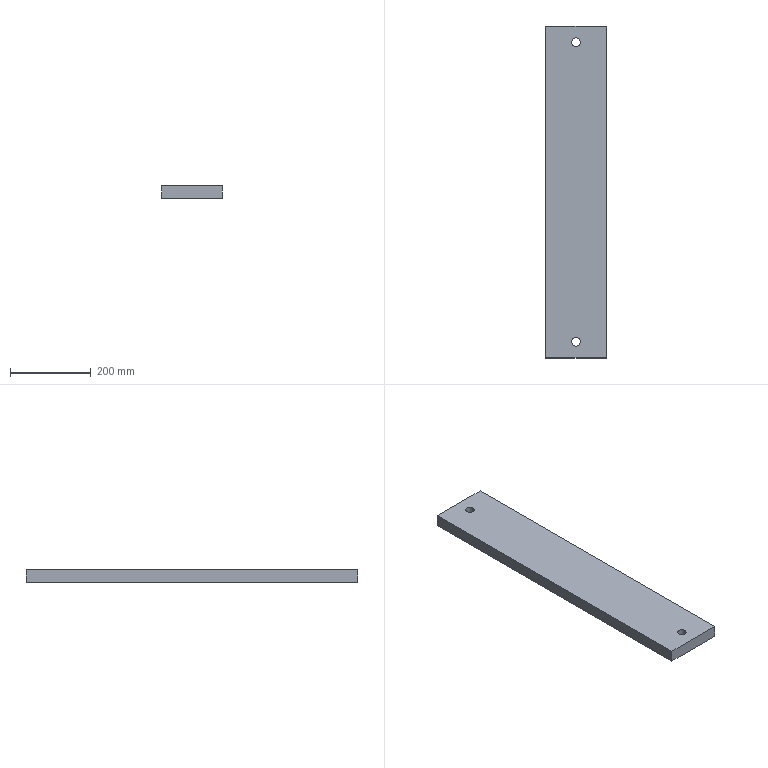Part | SolidWorks | features 3DProfileFeature 1, Extrusion 1, HoleWzd 1 | 1 solid | 10 faces | box 150 x 820 x 30 mm | volume 3669218 mm3 | plane 6 | cylinder 4 | commonest cylinder face diameters 21 x4
STEP:
#1=CARTESIAN_POINT('',(64.5,780.,0.));
#2=VERTEX_POINT('',#1);
#3=CARTESIAN_POINT('',(85.5,780.,0.));
#4=VERTEX_POINT('',#3);
#5=CARTESIAN_POINT('',(75.,780.,0.));
#6=DIRECTION('',(0.,0.,1.));
#7=DIRECTION('',(1.,0.,0.));
#8=AXIS2_PLACEMENT_3D('',#5,#6,#7);
#9=CIRCLE('',#8,10.5);
#10=EDGE_CURVE('',#2,#4,#9,.T.);
#11=ORIENTED_EDGE('',*,*,#10,.F.);
#12=CARTESIAN_POINT('',(64.5,780.,30.));
#13=VERTEX_POINT('',#12);
#14=CARTESIAN_POINT('',(64.5,780.,30.));
#15=DIRECTION('',(0.,0.,1.));
#16=VECTOR('',#15,1000.);
#17=LINE('',#14,#16);
#18=EDGE_CURVE('',#2,#13,#17,.T.);
#19=ORIENTED_EDGE('',*,*,#18,.T.);
#20=CARTESIAN_POINT('',(85.5,780.,30.));
#21=VERTEX_POINT('',#20);
#22=CARTESIAN_POINT('',(75.,780.,30.));
#23=DIRECTION('',(0.,0.,1.));
#24=DIRECTION('',(1.,0.,0.));
#25=AXIS2_PLACEMENT_3D('',#22,#23,#24);
#26=CIRCLE('',#25,10.5);
#27=EDGE_CURVE('',#13,#21,#26,.T.);
#28=ORIENTED_EDGE('',*,*,#27,.T.);
#29=CARTESIAN_POINT('',(85.5,780.,30.));
#30=DIRECTION('',(0.,0.,1.));
#31=VECTOR('',#30,1000.);
#32=LINE('',#29,#31);
#33=EDGE_CURVE('',#4,#21,#32,.T.);
#34=ORIENTED_EDGE('',*,*,#33,.F.);
#35=EDGE_LOOP('',(#11,#19,#28,#34));
#36=FACE_OUTER_BOUND('',#35,.T.);
#37=CARTESIAN_POINT('',(75.,780.,30.));
#38=DIRECTION('',(0.,0.,1.));
#39=DIRECTION('',(1.,0.,0.));
#40=AXIS2_PLACEMENT_3D('',#37,#38,#39);
#41=CYLINDRICAL_SURFACE('',#40,10.5);
#42=ADVANCED_FACE('',(#36),#41,.F.);
#43=CARTESIAN_POINT('',(64.5,40.,0.));
#44=VERTEX_POINT('',#43);
#45=CARTESIAN_POINT('',(85.5,40.,0.));
#46=VERTEX_POINT('',#45);
#47=CARTESIAN_POINT('',(75.,40.,0.));
#48=DIRECTION('',(0.,0.,1.));
#49=DIRECTION('',(1.,0.,0.));
#50=AXIS2_PLACEMENT_3D('',#47,#48,#49);
#51=CIRCLE('',#50,10.5);
#52=EDGE_CURVE('',#44,#46,#51,.T.);
#53=ORIENTED_EDGE('',*,*,#52,.F.);
#54=CARTESIAN_POINT('',(64.5,40.,30.));
#55=VERTEX_POINT('',#54);
#56=CARTESIAN_POINT('',(64.5,40.,30.));
#57=DIRECTION('',(0.,0.,1.));
#58=VECTOR('',#57,1000.);
#59=LINE('',#56,#58);
#60=EDGE_CURVE('',#44,#55,#59,.T.);
#61=ORIENTED_EDGE('',*,*,#60,.T.);
#62=CARTESIAN_POINT('',(85.5,40.,30.));
#63=VERTEX_POINT('',#62);
#64=CARTESIAN_POINT('',(75.,40.,30.));
#65=DIRECTION('',(0.,0.,1.));
#66=DIRECTION('',(1.,0.,0.));
#67=AXIS2_PLACEMENT_3D('',#64,#65,#66);
#68=CIRCLE('',#67,10.5);
#69=EDGE_CURVE('',#55,#63,#68,.T.);
#70=ORIENTED_EDGE('',*,*,#69,.T.);
#71=CARTESIAN_POINT('',(85.5,40.,30.));
#72=DIRECTION('',(0.,0.,1.));
#73=VECTOR('',#72,1000.);
#74=LINE('',#71,#73);
#75=EDGE_CURVE('',#46,#63,#74,.T.);
#76=ORIENTED_EDGE('',*,*,#75,.F.);
#77=EDGE_LOOP('',(#53,#61,#70,#76));
#78=FACE_OUTER_BOUND('',#77,.T.);
#79=CARTESIAN_POINT('',(75.,40.,30.));
#80=DIRECTION('',(0.,0.,1.));
#81=DIRECTION('',(1.,0.,0.));
#82=AXIS2_PLACEMENT_3D('',#79,#80,#81);
#83=CYLINDRICAL_SURFACE('',#82,10.5);
#84=ADVANCED_FACE('',(#78),#83,.F.);
#85=CARTESIAN_POINT('',(0.,820.,0.));
#86=VERTEX_POINT('',#85);
#87=CARTESIAN_POINT('',(0.,0.,0.));
#88=VERTEX_POINT('',#87);
#89=CARTESIAN_POINT('',(0.,0.,0.));
#90=DIRECTION('',(0.,-1.,0.));
#91=VECTOR('',#90,1000.);
#92=LINE('',#89,#91);
#93=EDGE_CURVE('',#86,#88,#92,.T.);
#94=ORIENTED_EDGE('',*,*,#93,.T.);
#95=CARTESIAN_POINT('',(0.,0.,30.));
#96=VERTEX_POINT('',#95);
#97=CARTESIAN_POINT('',(0.,0.,30.));
#98=DIRECTION('',(0.,0.,-1.));
#99=VECTOR('',#98,1000.);
#100=LINE('',#97,#99);
#101=EDGE_CURVE('',#96,#88,#100,.T.);
#102=ORIENTED_EDGE('',*,*,#101,.F.);
#103=CARTESIAN_POINT('',(0.,820.,30.));
#104=VERTEX_POINT('',#103);
#105=CARTESIAN_POINT('',(0.,0.,30.));
#106=DIRECTION('',(0.,-1.,0.));
#107=VECTOR('',#106,1000.);
#108=LINE('',#105,#107);
#109=EDGE_CURVE('',#104,#96,#108,.T.);
#110=ORIENTED_EDGE('',*,*,#109,.F.);
#111=CARTESIAN_POINT('',(0.,820.,30.));
#112=DIRECTION('',(0.,0.,-1.));
#113=VECTOR('',#112,1000.);
#114=LINE('',#111,#113);
#115=EDGE_CURVE('',#104,#86,#114,.T.);
#116=ORIENTED_EDGE('',*,*,#115,.T.);
#117=EDGE_LOOP('',(#94,#102,#110,#116));
#118=FACE_OUTER_BOUND('',#117,.T.);
#119=CARTESIAN_POINT('',(0.,0.,30.));
#120=DIRECTION('',(1.,0.,0.));
#121=DIRECTION('',(0.,0.,-1.));
#122=AXIS2_PLACEMENT_3D('',#119,#120,#121);
#123=PLANE('',#122);
#124=ADVANCED_FACE('',(#118),#123,.F.);
#125=CARTESIAN_POINT('',(150.,0.,0.));
#126=VERTEX_POINT('',#125);
#127=CARTESIAN_POINT('',(0.,0.,0.));
#128=DIRECTION('',(1.,0.,0.));
#129=VECTOR('',#128,1000.);
#130=LINE('',#127,#129);
#131=EDGE_CURVE('',#88,#126,#130,.T.);
#132=ORIENTED_EDGE('',*,*,#131,.T.);
#133=CARTESIAN_POINT('',(150.,0.,30.));
#134=VERTEX_POINT('',#133);
#135=CARTESIAN_POINT('',(150.,0.,30.));
#136=DIRECTION('',(0.,0.,-1.));
#137=VECTOR('',#136,1000.);
#138=LINE('',#135,#137);
#139=EDGE_CURVE('',#134,#126,#138,.T.);
#140=ORIENTED_EDGE('',*,*,#139,.F.);
#141=CARTESIAN_POINT('',(0.,0.,30.));
#142=DIRECTION('',(1.,0.,0.));
#143=VECTOR('',#142,1000.);
#144=LINE('',#141,#143);
#145=EDGE_CURVE('',#96,#134,#144,.T.);
#146=ORIENTED_EDGE('',*,*,#145,.F.);
#147=ORIENTED_EDGE('',*,*,#101,.T.);
#148=EDGE_LOOP('',(#132,#140,#146,#147));
#149=FACE_OUTER_BOUND('',#148,.T.);
#150=CARTESIAN_POINT('',(0.,0.,30.));
#151=DIRECTION('',(0.,1.,0.));
#152=DIRECTION('',(0.,0.,1.));
#153=AXIS2_PLACEMENT_3D('',#150,#151,#152);
#154=PLANE('',#153);
#155=ADVANCED_FACE('',(#149),#154,.F.);
#156=CARTESIAN_POINT('',(150.,820.,0.));
#157=VERTEX_POINT('',#156);
#158=CARTESIAN_POINT('',(150.,0.,0.));
#159=DIRECTION('',(0.,1.,0.));
#160=VECTOR('',#159,1000.);
#161=LINE('',#158,#160);
#162=EDGE_CURVE('',#126,#157,#161,.T.);
#163=ORIENTED_EDGE('',*,*,#162,.T.);
#164=CARTESIAN_POINT('',(150.,820.,30.));
#165=VERTEX_POINT('',#164);
#166=CARTESIAN_POINT('',(150.,820.,30.));
#167=DIRECTION('',(0.,0.,-1.));
#168=VECTOR('',#167,1000.);
#169=LINE('',#166,#168);
#170=EDGE_CURVE('',#165,#157,#169,.T.);
#171=ORIENTED_EDGE('',*,*,#170,.F.);
#172=CARTESIAN_POINT('',(150.,0.,30.));
#173=DIRECTION('',(0.,1.,0.));
#174=VECTOR('',#173,1000.);
#175=LINE('',#172,#174);
#176=EDGE_CURVE('',#134,#165,#175,.T.);
#177=ORIENTED_EDGE('',*,*,#176,.F.);
#178=ORIENTED_EDGE('',*,*,#139,.T.);
#179=EDGE_LOOP('',(#163,#171,#177,#178));
#180=FACE_OUTER_BOUND('',#179,.T.);
#181=CARTESIAN_POINT('',(150.,0.,30.));
#182=DIRECTION('',(-1.,0.,0.));
#183=DIRECTION('',(0.,0.,1.));
#184=AXIS2_PLACEMENT_3D('',#181,#182,#183);
#185=PLANE('',#184);
#186=ADVANCED_FACE('',(#180),#185,.F.);
#187=CARTESIAN_POINT('',(0.,820.,0.));
#188=DIRECTION('',(-1.,0.,0.));
#189=VECTOR('',#188,1000.);
#190=LINE('',#187,#189);
#191=EDGE_CURVE('',#157,#86,#190,.T.);
#192=ORIENTED_EDGE('',*,*,#191,.T.);
#193=ORIENTED_EDGE('',*,*,#115,.F.);
#194=CARTESIAN_POINT('',(0.,820.,30.));
#195=DIRECTION('',(-1.,0.,0.));
#196=VECTOR('',#195,1000.);
#197=LINE('',#194,#196);
#198=EDGE_CURVE('',#165,#104,#197,.T.);
#199=ORIENTED_EDGE('',*,*,#198,.F.);
#200=ORIENTED_EDGE('',*,*,#170,.T.);
#201=EDGE_LOOP('',(#192,#193,#199,#200));
#202=FACE_OUTER_BOUND('',#201,.T.);
#203=CARTESIAN_POINT('',(0.,820.,30.));
#204=DIRECTION('',(0.,-1.,0.));
#205=DIRECTION('',(0.,0.,-1.));
#206=AXIS2_PLACEMENT_3D('',#203,#204,#205);
#207=PLANE('',#206);
#208=ADVANCED_FACE('',(#202),#207,.F.);
#209=CARTESIAN_POINT('',(75.,780.,30.));
#210=DIRECTION('',(0.,0.,1.));
#211=DIRECTION('',(1.,0.,0.));
#212=AXIS2_PLACEMENT_3D('',#209,#210,#211);
#213=CIRCLE('',#212,10.5);
#214=EDGE_CURVE('',#21,#13,#213,.T.);
#215=ORIENTED_EDGE('',*,*,#214,.F.);
#216=ORIENTED_EDGE('',*,*,#27,.F.);
#217=EDGE_LOOP('',(#215,#216));
#218=FACE_BOUND('',#217,.T.);
#219=CARTESIAN_POINT('',(75.,40.,30.));
#220=DIRECTION('',(0.,0.,1.));
#221=DIRECTION('',(1.,0.,0.));
#222=AXIS2_PLACEMENT_3D('',#219,#220,#221);
#223=CIRCLE('',#222,10.5);
#224=EDGE_CURVE('',#63,#55,#223,.T.);
#225=ORIENTED_EDGE('',*,*,#224,.F.);
#226=ORIENTED_EDGE('',*,*,#69,.F.);
#227=EDGE_LOOP('',(#225,#226));
#228=FACE_BOUND('',#227,.T.);
#229=ORIENTED_EDGE('',*,*,#109,.T.);
#230=ORIENTED_EDGE('',*,*,#145,.T.);
#231=ORIENTED_EDGE('',*,*,#176,.T.);
#232=ORIENTED_EDGE('',*,*,#198,.T.);
#233=EDGE_LOOP('',(#229,#230,#231,#232));
#234=FACE_OUTER_BOUND('',#233,.T.);
#235=CARTESIAN_POINT('',(0.,0.,30.));
#236=DIRECTION('',(0.,0.,-1.));
#237=DIRECTION('',(-1.,0.,0.));
#238=AXIS2_PLACEMENT_3D('',#235,#236,#237);
#239=PLANE('',#238);
#240=ADVANCED_FACE('',(#218,#228,#234),#239,.F.);
#241=CARTESIAN_POINT('',(75.,780.,0.));
#242=DIRECTION('',(0.,0.,1.));
#243=DIRECTION('',(1.,0.,0.));
#244=AXIS2_PLACEMENT_3D('',#241,#242,#243);
#245=CIRCLE('',#244,10.5);
#246=EDGE_CURVE('',#4,#2,#245,.T.);
#247=ORIENTED_EDGE('',*,*,#246,.T.);
#248=ORIENTED_EDGE('',*,*,#10,.T.);
#249=EDGE_LOOP('',(#247,#248));
#250=FACE_BOUND('',#249,.T.);
#251=CARTESIAN_POINT('',(75.,40.,0.));
#252=DIRECTION('',(0.,0.,1.));
#253=DIRECTION('',(1.,0.,0.));
#254=AXIS2_PLACEMENT_3D('',#251,#252,#253);
#255=CIRCLE('',#254,10.5);
#256=EDGE_CURVE('',#46,#44,#255,.T.);
#257=ORIENTED_EDGE('',*,*,#256,.T.);
#258=ORIENTED_EDGE('',*,*,#52,.T.);
#259=EDGE_LOOP('',(#257,#258));
#260=FACE_BOUND('',#259,.T.);
#261=ORIENTED_EDGE('',*,*,#93,.F.);
#262=ORIENTED_EDGE('',*,*,#191,.F.);
#263=ORIENTED_EDGE('',*,*,#162,.F.);
#264=ORIENTED_EDGE('',*,*,#131,.F.);
#265=EDGE_LOOP('',(#261,#262,#263,#264));
#266=FACE_OUTER_BOUND('',#265,.T.);
#267=CARTESIAN_POINT('',(0.,0.,0.));
#268=DIRECTION('',(0.,0.,-1.));
#269=DIRECTION('',(-1.,0.,0.));
#270=AXIS2_PLACEMENT_3D('',#267,#268,#269);
#271=PLANE('',#270);
#272=ADVANCED_FACE('',(#250,#260,#266),#271,.T.);
#273=ORIENTED_EDGE('',*,*,#60,.F.);
#274=ORIENTED_EDGE('',*,*,#256,.F.);
#275=ORIENTED_EDGE('',*,*,#75,.T.);
#276=ORIENTED_EDGE('',*,*,#224,.T.);
#277=EDGE_LOOP('',(#273,#274,#275,#276));
#278=FACE_OUTER_BOUND('',#277,.T.);
#279=CARTESIAN_POINT('',(75.,40.,30.));
#280=DIRECTION('',(0.,0.,1.));
#281=DIRECTION('',(1.,0.,0.));
#282=AXIS2_PLACEMENT_3D('',#279,#280,#281);
#283=CYLINDRICAL_SURFACE('',#282,10.5);
#284=ADVANCED_FACE('',(#278),#283,.F.);
#285=ORIENTED_EDGE('',*,*,#18,.F.);
#286=ORIENTED_EDGE('',*,*,#246,.F.);
#287=ORIENTED_EDGE('',*,*,#33,.T.);
#288=ORIENTED_EDGE('',*,*,#214,.T.);
#289=EDGE_LOOP('',(#285,#286,#287,#288));
#290=FACE_OUTER_BOUND('',#289,.T.);
#291=CARTESIAN_POINT('',(75.,780.,30.));
#292=DIRECTION('',(0.,0.,1.));
#293=DIRECTION('',(1.,0.,0.));
#294=AXIS2_PLACEMENT_3D('',#291,#292,#293);
#295=CYLINDRICAL_SURFACE('',#294,10.5);
#296=ADVANCED_FACE('',(#290),#295,.F.);
#297=CLOSED_SHELL('',(#42,#84,#124,#155,#186,#208,#240,#272,#284,#296));
#298=MANIFOLD_SOLID_BREP('',#297);
#299=CARTESIAN_POINT('',(0.,0.,0.));
#300=DIRECTION('',(0.,0.,1.));
#301=DIRECTION('',(1.,0.,0.));
#302=AXIS2_PLACEMENT_3D('',#299,#300,#301);
#303=(LENGTH_UNIT()NAMED_UNIT(*)SI_UNIT(.MILLI.,.METRE.));
#304=UNCERTAINTY_MEASURE_WITH_UNIT(LENGTH_MEASURE(0.00001),#303,'','');
#305=(NAMED_UNIT(*)PLANE_ANGLE_UNIT()SI_UNIT($,.RADIAN.));
#306=(NAMED_UNIT(*)SI_UNIT($,.STERADIAN.)SOLID_ANGLE_UNIT());
#307=(GEOMETRIC_REPRESENTATION_CONTEXT(3)GLOBAL_UNCERTAINTY_ASSIGNED_CONTEXT((#304))GLOBAL_UNIT_ASSIGNED_CONTEXT((#303,#305,#306))REPRESENTATION_CONTEXT('',''));
#308=ADVANCED_BREP_SHAPE_REPRESENTATION('',(#298,#302),#307);